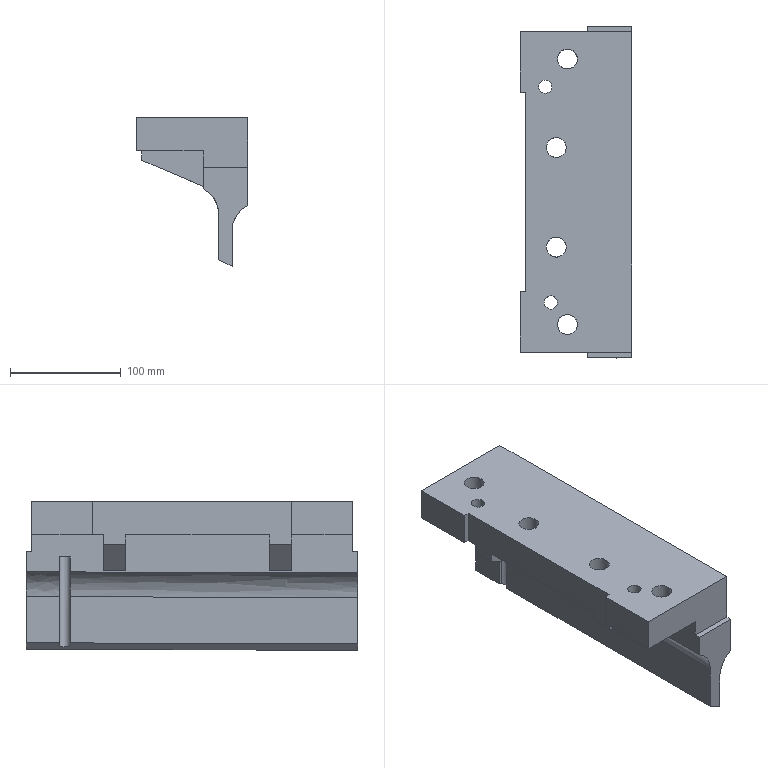Part | NX | features solid 2 | 1 solid | 48 faces | box 100.514 x 300 x 134.44 mm | volume 1590567 mm3 | plane 28 | cylinder 11 | spline 9 | commonest cylinder face diameters 18 x4 26 x4 12 x2 10 x1